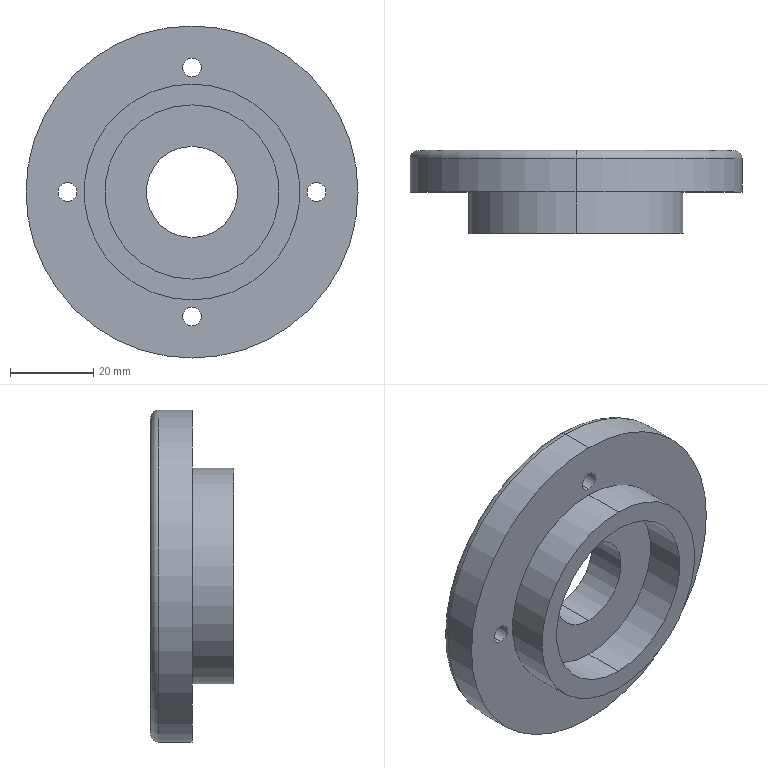Part | SolidWorks | features ICE 2, CirPattern 1, Extrusion 1, Fillet 1, HoleWzd 1 | 1 solid | 34 faces | box 80 x 20 x 80 mm | volume 52365 mm3 | cylinder 24 | plane 8 | torus 2 | commonest cylinder face diameters 4.5 x8 8 x8 22 x2 42 x2 52 x2 80 x2
STEP:
#1=CARTESIAN_POINT('',(-30.,15.4,-4.));
#2=VERTEX_POINT('',#1);
#3=CARTESIAN_POINT('',(-30.,15.4,4.));
#4=VERTEX_POINT('',#3);
#5=CARTESIAN_POINT('',(-30.,15.4,0.));
#6=DIRECTION('',(0.,1.,0.));
#7=DIRECTION('',(0.,0.,1.));
#8=AXIS2_PLACEMENT_3D('',#5,#6,#7);
#9=CIRCLE('',#8,4.);
#10=EDGE_CURVE('',#2,#4,#9,.T.);
#11=ORIENTED_EDGE('',*,*,#10,.F.);
#12=CARTESIAN_POINT('',(-30.,20.,-4.));
#13=VERTEX_POINT('',#12);
#14=CARTESIAN_POINT('',(-30.,20.,-4.));
#15=DIRECTION('',(0.,1.,0.));
#16=VECTOR('',#15,1000.);
#17=LINE('',#14,#16);
#18=EDGE_CURVE('',#2,#13,#17,.T.);
#19=ORIENTED_EDGE('',*,*,#18,.T.);
#20=CARTESIAN_POINT('',(-30.,20.,4.));
#21=VERTEX_POINT('',#20);
#22=CARTESIAN_POINT('',(-30.,20.,0.));
#23=DIRECTION('',(0.,1.,0.));
#24=DIRECTION('',(0.,0.,1.));
#25=AXIS2_PLACEMENT_3D('',#22,#23,#24);
#26=CIRCLE('',#25,4.);
#27=EDGE_CURVE('',#13,#21,#26,.T.);
#28=ORIENTED_EDGE('',*,*,#27,.T.);
#29=CARTESIAN_POINT('',(-30.,20.,4.));
#30=DIRECTION('',(0.,1.,0.));
#31=VECTOR('',#30,1000.);
#32=LINE('',#29,#31);
#33=EDGE_CURVE('',#4,#21,#32,.T.);
#34=ORIENTED_EDGE('',*,*,#33,.F.);
#35=EDGE_LOOP('',(#11,#19,#28,#34));
#36=FACE_OUTER_BOUND('',#35,.T.);
#37=CARTESIAN_POINT('',(-30.,20.,0.));
#38=DIRECTION('',(0.,1.,0.));
#39=DIRECTION('',(0.,0.,1.));
#40=AXIS2_PLACEMENT_3D('',#37,#38,#39);
#41=CYLINDRICAL_SURFACE('',#40,4.);
#42=ADVANCED_FACE('',(#36),#41,.F.);
#43=CARTESIAN_POINT('',(-30.,10.,-2.25));
#44=VERTEX_POINT('',#43);
#45=CARTESIAN_POINT('',(-30.,10.,2.25));
#46=VERTEX_POINT('',#45);
#47=CARTESIAN_POINT('',(-30.,10.,0.));
#48=DIRECTION('',(0.,1.,0.));
#49=DIRECTION('',(0.,0.,1.));
#50=AXIS2_PLACEMENT_3D('',#47,#48,#49);
#51=CIRCLE('',#50,2.25);
#52=EDGE_CURVE('',#44,#46,#51,.T.);
#53=ORIENTED_EDGE('',*,*,#52,.F.);
#54=CARTESIAN_POINT('',(-30.,15.4,-2.25));
#55=VERTEX_POINT('',#54);
#56=CARTESIAN_POINT('',(-30.,20.,-2.25));
#57=DIRECTION('',(0.,1.,0.));
#58=VECTOR('',#57,1000.);
#59=LINE('',#56,#58);
#60=EDGE_CURVE('',#44,#55,#59,.T.);
#61=ORIENTED_EDGE('',*,*,#60,.T.);
#62=CARTESIAN_POINT('',(-30.,15.4,2.25));
#63=VERTEX_POINT('',#62);
#64=CARTESIAN_POINT('',(-30.,15.4,0.));
#65=DIRECTION('',(0.,1.,0.));
#66=DIRECTION('',(0.,0.,1.));
#67=AXIS2_PLACEMENT_3D('',#64,#65,#66);
#68=CIRCLE('',#67,2.25);
#69=EDGE_CURVE('',#55,#63,#68,.T.);
#70=ORIENTED_EDGE('',*,*,#69,.T.);
#71=CARTESIAN_POINT('',(-30.,20.,2.25));
#72=DIRECTION('',(0.,1.,0.));
#73=VECTOR('',#72,1000.);
#74=LINE('',#71,#73);
#75=EDGE_CURVE('',#46,#63,#74,.T.);
#76=ORIENTED_EDGE('',*,*,#75,.F.);
#77=EDGE_LOOP('',(#53,#61,#70,#76));
#78=FACE_OUTER_BOUND('',#77,.T.);
#79=CARTESIAN_POINT('',(-30.,20.,0.));
#80=DIRECTION('',(0.,1.,0.));
#81=DIRECTION('',(0.,0.,1.));
#82=AXIS2_PLACEMENT_3D('',#79,#80,#81);
#83=CYLINDRICAL_SURFACE('',#82,2.25);
#84=ADVANCED_FACE('',(#78),#83,.F.);
#85=CARTESIAN_POINT('',(0.,15.4,26.));
#86=VERTEX_POINT('',#85);
#87=CARTESIAN_POINT('',(0.,15.4,34.));
#88=VERTEX_POINT('',#87);
#89=CARTESIAN_POINT('',(0.,15.4,30.));
#90=DIRECTION('',(0.,1.,0.));
#91=DIRECTION('',(0.,0.,1.));
#92=AXIS2_PLACEMENT_3D('',#89,#90,#91);
#93=CIRCLE('',#92,4.);
#94=EDGE_CURVE('',#86,#88,#93,.T.);
#95=ORIENTED_EDGE('',*,*,#94,.F.);
#96=CARTESIAN_POINT('',(0.,20.,26.));
#97=VERTEX_POINT('',#96);
#98=CARTESIAN_POINT('',(0.,20.,26.));
#99=DIRECTION('',(0.,1.,0.));
#100=VECTOR('',#99,1000.);
#101=LINE('',#98,#100);
#102=EDGE_CURVE('',#86,#97,#101,.T.);
#103=ORIENTED_EDGE('',*,*,#102,.T.);
#104=CARTESIAN_POINT('',(0.,20.,34.));
#105=VERTEX_POINT('',#104);
#106=CARTESIAN_POINT('',(0.,20.,30.));
#107=DIRECTION('',(0.,1.,0.));
#108=DIRECTION('',(0.,0.,1.));
#109=AXIS2_PLACEMENT_3D('',#106,#107,#108);
#110=CIRCLE('',#109,4.);
#111=EDGE_CURVE('',#97,#105,#110,.T.);
#112=ORIENTED_EDGE('',*,*,#111,.T.);
#113=CARTESIAN_POINT('',(0.,20.,34.));
#114=DIRECTION('',(0.,1.,0.));
#115=VECTOR('',#114,1000.);
#116=LINE('',#113,#115);
#117=EDGE_CURVE('',#88,#105,#116,.T.);
#118=ORIENTED_EDGE('',*,*,#117,.F.);
#119=EDGE_LOOP('',(#95,#103,#112,#118));
#120=FACE_OUTER_BOUND('',#119,.T.);
#121=CARTESIAN_POINT('',(0.,20.,30.));
#122=DIRECTION('',(0.,1.,0.));
#123=DIRECTION('',(0.,0.,1.));
#124=AXIS2_PLACEMENT_3D('',#121,#122,#123);
#125=CYLINDRICAL_SURFACE('',#124,4.);
#126=ADVANCED_FACE('',(#120),#125,.F.);
#127=CARTESIAN_POINT('',(0.,10.,27.75));
#128=VERTEX_POINT('',#127);
#129=CARTESIAN_POINT('',(0.,10.,32.25));
#130=VERTEX_POINT('',#129);
#131=CARTESIAN_POINT('',(0.,10.,30.));
#132=DIRECTION('',(0.,1.,0.));
#133=DIRECTION('',(0.,0.,1.));
#134=AXIS2_PLACEMENT_3D('',#131,#132,#133);
#135=CIRCLE('',#134,2.25);
#136=EDGE_CURVE('',#128,#130,#135,.T.);
#137=ORIENTED_EDGE('',*,*,#136,.F.);
#138=CARTESIAN_POINT('',(0.,15.4,27.75));
#139=VERTEX_POINT('',#138);
#140=CARTESIAN_POINT('',(0.,20.,27.75));
#141=DIRECTION('',(0.,1.,0.));
#142=VECTOR('',#141,1000.);
#143=LINE('',#140,#142);
#144=EDGE_CURVE('',#128,#139,#143,.T.);
#145=ORIENTED_EDGE('',*,*,#144,.T.);
#146=CARTESIAN_POINT('',(0.,15.4,32.25));
#147=VERTEX_POINT('',#146);
#148=CARTESIAN_POINT('',(0.,15.4,30.));
#149=DIRECTION('',(0.,1.,0.));
#150=DIRECTION('',(0.,0.,1.));
#151=AXIS2_PLACEMENT_3D('',#148,#149,#150);
#152=CIRCLE('',#151,2.25);
#153=EDGE_CURVE('',#139,#147,#152,.T.);
#154=ORIENTED_EDGE('',*,*,#153,.T.);
#155=CARTESIAN_POINT('',(0.,20.,32.25));
#156=DIRECTION('',(0.,1.,0.));
#157=VECTOR('',#156,1000.);
#158=LINE('',#155,#157);
#159=EDGE_CURVE('',#130,#147,#158,.T.);
#160=ORIENTED_EDGE('',*,*,#159,.F.);
#161=EDGE_LOOP('',(#137,#145,#154,#160));
#162=FACE_OUTER_BOUND('',#161,.T.);
#163=CARTESIAN_POINT('',(0.,20.,30.));
#164=DIRECTION('',(0.,1.,0.));
#165=DIRECTION('',(0.,0.,1.));
#166=AXIS2_PLACEMENT_3D('',#163,#164,#165);
#167=CYLINDRICAL_SURFACE('',#166,2.25);
#168=ADVANCED_FACE('',(#162),#167,.F.);
#169=CARTESIAN_POINT('',(30.,15.4,-4.));
#170=VERTEX_POINT('',#169);
#171=CARTESIAN_POINT('',(30.,15.4,4.));
#172=VERTEX_POINT('',#171);
#173=CARTESIAN_POINT('',(30.,15.4,0.));
#174=DIRECTION('',(0.,1.,0.));
#175=DIRECTION('',(0.,0.,1.));
#176=AXIS2_PLACEMENT_3D('',#173,#174,#175);
#177=CIRCLE('',#176,4.);
#178=EDGE_CURVE('',#170,#172,#177,.T.);
#179=ORIENTED_EDGE('',*,*,#178,.F.);
#180=CARTESIAN_POINT('',(30.,20.,-4.));
#181=VERTEX_POINT('',#180);
#182=CARTESIAN_POINT('',(30.,20.,-4.));
#183=DIRECTION('',(0.,1.,0.));
#184=VECTOR('',#183,1000.);
#185=LINE('',#182,#184);
#186=EDGE_CURVE('',#170,#181,#185,.T.);
#187=ORIENTED_EDGE('',*,*,#186,.T.);
#188=CARTESIAN_POINT('',(30.,20.,4.));
#189=VERTEX_POINT('',#188);
#190=CARTESIAN_POINT('',(30.,20.,0.));
#191=DIRECTION('',(0.,1.,0.));
#192=DIRECTION('',(0.,0.,1.));
#193=AXIS2_PLACEMENT_3D('',#190,#191,#192);
#194=CIRCLE('',#193,4.);
#195=EDGE_CURVE('',#181,#189,#194,.T.);
#196=ORIENTED_EDGE('',*,*,#195,.T.);
#197=CARTESIAN_POINT('',(30.,20.,4.));
#198=DIRECTION('',(0.,1.,0.));
#199=VECTOR('',#198,1000.);
#200=LINE('',#197,#199);
#201=EDGE_CURVE('',#172,#189,#200,.T.);
#202=ORIENTED_EDGE('',*,*,#201,.F.);
#203=EDGE_LOOP('',(#179,#187,#196,#202));
#204=FACE_OUTER_BOUND('',#203,.T.);
#205=CARTESIAN_POINT('',(30.,20.,0.));
#206=DIRECTION('',(0.,1.,0.));
#207=DIRECTION('',(0.,0.,1.));
#208=AXIS2_PLACEMENT_3D('',#205,#206,#207);
#209=CYLINDRICAL_SURFACE('',#208,4.);
#210=ADVANCED_FACE('',(#204),#209,.F.);
#211=CARTESIAN_POINT('',(30.,10.,-2.25));
#212=VERTEX_POINT('',#211);
#213=CARTESIAN_POINT('',(30.,10.,2.25));
#214=VERTEX_POINT('',#213);
#215=CARTESIAN_POINT('',(30.,10.,0.));
#216=DIRECTION('',(0.,1.,0.));
#217=DIRECTION('',(0.,0.,1.));
#218=AXIS2_PLACEMENT_3D('',#215,#216,#217);
#219=CIRCLE('',#218,2.25);
#220=EDGE_CURVE('',#212,#214,#219,.T.);
#221=ORIENTED_EDGE('',*,*,#220,.F.);
#222=CARTESIAN_POINT('',(30.,15.4,-2.25));
#223=VERTEX_POINT('',#222);
#224=CARTESIAN_POINT('',(30.,20.,-2.25));
#225=DIRECTION('',(0.,1.,0.));
#226=VECTOR('',#225,1000.);
#227=LINE('',#224,#226);
#228=EDGE_CURVE('',#212,#223,#227,.T.);
#229=ORIENTED_EDGE('',*,*,#228,.T.);
#230=CARTESIAN_POINT('',(30.,15.4,2.25));
#231=VERTEX_POINT('',#230);
#232=CARTESIAN_POINT('',(30.,15.4,0.));
#233=DIRECTION('',(0.,1.,0.));
#234=DIRECTION('',(0.,0.,1.));
#235=AXIS2_PLACEMENT_3D('',#232,#233,#234);
#236=CIRCLE('',#235,2.25);
#237=EDGE_CURVE('',#223,#231,#236,.T.);
#238=ORIENTED_EDGE('',*,*,#237,.T.);
#239=CARTESIAN_POINT('',(30.,20.,2.25));
#240=DIRECTION('',(0.,1.,0.));
#241=VECTOR('',#240,1000.);
#242=LINE('',#239,#241);
#243=EDGE_CURVE('',#214,#231,#242,.T.);
#244=ORIENTED_EDGE('',*,*,#243,.F.);
#245=EDGE_LOOP('',(#221,#229,#238,#244));
#246=FACE_OUTER_BOUND('',#245,.T.);
#247=CARTESIAN_POINT('',(30.,20.,0.));
#248=DIRECTION('',(0.,1.,0.));
#249=DIRECTION('',(0.,0.,1.));
#250=AXIS2_PLACEMENT_3D('',#247,#248,#249);
#251=CYLINDRICAL_SURFACE('',#250,2.25);
#252=ADVANCED_FACE('',(#246),#251,.F.);
#253=CARTESIAN_POINT('',(0.,15.4,-34.));
#254=VERTEX_POINT('',#253);
#255=CARTESIAN_POINT('',(0.,15.4,-26.));
#256=VERTEX_POINT('',#255);
#257=CARTESIAN_POINT('',(0.,15.4,-30.));
#258=DIRECTION('',(0.,1.,0.));
#259=DIRECTION('',(0.,0.,1.));
#260=AXIS2_PLACEMENT_3D('',#257,#258,#259);
#261=CIRCLE('',#260,4.);
#262=EDGE_CURVE('',#254,#256,#261,.T.);
#263=ORIENTED_EDGE('',*,*,#262,.F.);
#264=CARTESIAN_POINT('',(0.,20.,-34.));
#265=VERTEX_POINT('',#264);
#266=CARTESIAN_POINT('',(0.,20.,-34.));
#267=DIRECTION('',(0.,1.,0.));
#268=VECTOR('',#267,1000.);
#269=LINE('',#266,#268);
#270=EDGE_CURVE('',#254,#265,#269,.T.);
#271=ORIENTED_EDGE('',*,*,#270,.T.);
#272=CARTESIAN_POINT('',(0.,20.,-26.));
#273=VERTEX_POINT('',#272);
#274=CARTESIAN_POINT('',(0.,20.,-30.));
#275=DIRECTION('',(0.,1.,0.));
#276=DIRECTION('',(0.,0.,1.));
#277=AXIS2_PLACEMENT_3D('',#274,#275,#276);
#278=CIRCLE('',#277,4.);
#279=EDGE_CURVE('',#265,#273,#278,.T.);
#280=ORIENTED_EDGE('',*,*,#279,.T.);
#281=CARTESIAN_POINT('',(0.,20.,-26.));
#282=DIRECTION('',(0.,1.,0.));
#283=VECTOR('',#282,1000.);
#284=LINE('',#281,#283);
#285=EDGE_CURVE('',#256,#273,#284,.T.);
#286=ORIENTED_EDGE('',*,*,#285,.F.);
#287=EDGE_LOOP('',(#263,#271,#280,#286));
#288=FACE_OUTER_BOUND('',#287,.T.);
#289=CARTESIAN_POINT('',(0.,20.,-30.));
#290=DIRECTION('',(0.,1.,0.));
#291=DIRECTION('',(0.,0.,1.));
#292=AXIS2_PLACEMENT_3D('',#289,#290,#291);
#293=CYLINDRICAL_SURFACE('',#292,4.);
#294=ADVANCED_FACE('',(#288),#293,.F.);
#295=CARTESIAN_POINT('',(0.,10.,-32.25));
#296=VERTEX_POINT('',#295);
#297=CARTESIAN_POINT('',(0.,10.,-27.75));
#298=VERTEX_POINT('',#297);
#299=CARTESIAN_POINT('',(0.,10.,-30.));
#300=DIRECTION('',(0.,1.,0.));
#301=DIRECTION('',(0.,0.,1.));
#302=AXIS2_PLACEMENT_3D('',#299,#300,#301);
#303=CIRCLE('',#302,2.25);
#304=EDGE_CURVE('',#296,#298,#303,.T.);
#305=ORIENTED_EDGE('',*,*,#304,.F.);
#306=CARTESIAN_POINT('',(0.,15.4,-32.25));
#307=VERTEX_POINT('',#306);
#308=CARTESIAN_POINT('',(0.,20.,-32.25));
#309=DIRECTION('',(0.,1.,0.));
#310=VECTOR('',#309,1000.);
#311=LINE('',#308,#310);
#312=EDGE_CURVE('',#296,#307,#311,.T.);
#313=ORIENTED_EDGE('',*,*,#312,.T.);
#314=CARTESIAN_POINT('',(0.,15.4,-27.75));
#315=VERTEX_POINT('',#314);
#316=CARTESIAN_POINT('',(0.,15.4,-30.));
#317=DIRECTION('',(0.,1.,0.));
#318=DIRECTION('',(0.,0.,1.));
#319=AXIS2_PLACEMENT_3D('',#316,#317,#318);
#320=CIRCLE('',#319,2.25);
#321=EDGE_CURVE('',#307,#315,#320,.T.);
#322=ORIENTED_EDGE('',*,*,#321,.T.);
#323=CARTESIAN_POINT('',(0.,20.,-27.75));
#324=DIRECTION('',(0.,1.,0.));
#325=VECTOR('',#324,1000.);
#326=LINE('',#323,#325);
#327=EDGE_CURVE('',#298,#315,#326,.T.);
#328=ORIENTED_EDGE('',*,*,#327,.F.);
#329=EDGE_LOOP('',(#305,#313,#322,#328));
#330=FACE_OUTER_BOUND('',#329,.T.);
#331=CARTESIAN_POINT('',(0.,20.,-30.));
#332=DIRECTION('',(0.,1.,0.));
#333=DIRECTION('',(0.,0.,1.));
#334=AXIS2_PLACEMENT_3D('',#331,#332,#333);
#335=CYLINDRICAL_SURFACE('',#334,2.25);
#336=ADVANCED_FACE('',(#330),#335,.F.);
#337=CARTESIAN_POINT('',(0.,18.,-40.));
#338=VERTEX_POINT('',#337);
#339=CARTESIAN_POINT('',(0.,18.,40.));
#340=VERTEX_POINT('',#339);
#341=CARTESIAN_POINT('',(0.,18.,0.));
#342=DIRECTION('',(0.,-1.,0.));
#343=DIRECTION('',(0.,0.,1.));
#344=AXIS2_PLACEMENT_3D('',#341,#342,#343);
#345=CIRCLE('',#344,40.);
#346=EDGE_CURVE('',#338,#340,#345,.T.);
#347=ORIENTED_EDGE('',*,*,#346,.F.);
#348=CARTESIAN_POINT('',(0.,20.,-38.));
#349=VERTEX_POINT('',#348);
#350=CARTESIAN_POINT('',(0.,18.,-38.));
#351=DIRECTION('',(1.,0.,0.));
#352=DIRECTION('',(0.,0.,-1.));
#353=AXIS2_PLACEMENT_3D('',#350,#351,#352);
#354=CIRCLE('',#353,2.);
#355=EDGE_CURVE('',#338,#349,#354,.T.);
#356=ORIENTED_EDGE('',*,*,#355,.T.);
#357=CARTESIAN_POINT('',(0.,20.,38.));
#358=VERTEX_POINT('',#357);
#359=CARTESIAN_POINT('',(0.,20.,0.));
#360=DIRECTION('',(0.,1.,0.));
#361=DIRECTION('',(0.,0.,1.));
#362=AXIS2_PLACEMENT_3D('',#359,#360,#361);
#363=CIRCLE('',#362,38.);
#364=EDGE_CURVE('',#358,#349,#363,.T.);
#365=ORIENTED_EDGE('',*,*,#364,.F.);
#366=CARTESIAN_POINT('',(0.,18.,38.));
#367=DIRECTION('',(-1.,0.,0.));
#368=DIRECTION('',(0.,0.,1.));
#369=AXIS2_PLACEMENT_3D('',#366,#367,#368);
#370=CIRCLE('',#369,2.);
#371=EDGE_CURVE('',#340,#358,#370,.T.);
#372=ORIENTED_EDGE('',*,*,#371,.F.);
#373=EDGE_LOOP('',(#347,#356,#365,#372));
#374=FACE_OUTER_BOUND('',#373,.T.);
#375=CARTESIAN_POINT('',(0.,18.,0.));
#376=DIRECTION('',(0.,1.,0.));
#377=DIRECTION('',(0.,0.,1.));
#378=AXIS2_PLACEMENT_3D('',#375,#376,#377);
#379=TOROIDAL_SURFACE('',#378,38.,2.);
#380=ADVANCED_FACE('',(#374),#379,.T.);
#381=CARTESIAN_POINT('',(0.,20.,11.));
#382=VERTEX_POINT('',#381);
#383=CARTESIAN_POINT('',(0.,20.,-11.));
#384=VERTEX_POINT('',#383);
#385=CARTESIAN_POINT('',(0.,20.,0.));
#386=DIRECTION('',(0.,-1.,0.));
#387=DIRECTION('',(0.,0.,-1.));
#388=AXIS2_PLACEMENT_3D('',#385,#386,#387);
#389=CIRCLE('',#388,11.);
#390=EDGE_CURVE('',#382,#384,#389,.T.);
#391=ORIENTED_EDGE('',*,*,#390,.F.);
#392=CARTESIAN_POINT('',(0.,10.,11.));
#393=VERTEX_POINT('',#392);
#394=CARTESIAN_POINT('',(0.,20.,11.));
#395=DIRECTION('',(0.,-1.,0.));
#396=VECTOR('',#395,1000.);
#397=LINE('',#394,#396);
#398=EDGE_CURVE('',#382,#393,#397,.T.);
#399=ORIENTED_EDGE('',*,*,#398,.T.);
#400=CARTESIAN_POINT('',(0.,10.,-11.));
#401=VERTEX_POINT('',#400);
#402=CARTESIAN_POINT('',(0.,10.,0.));
#403=DIRECTION('',(0.,-1.,0.));
#404=DIRECTION('',(0.,0.,-1.));
#405=AXIS2_PLACEMENT_3D('',#402,#403,#404);
#406=CIRCLE('',#405,11.);
#407=EDGE_CURVE('',#393,#401,#406,.T.);
#408=ORIENTED_EDGE('',*,*,#407,.T.);
#409=CARTESIAN_POINT('',(0.,20.,-11.));
#410=DIRECTION('',(0.,-1.,0.));
#411=VECTOR('',#410,1000.);
#412=LINE('',#409,#411);
#413=EDGE_CURVE('',#384,#401,#412,.T.);
#414=ORIENTED_EDGE('',*,*,#413,.F.);
#415=EDGE_LOOP('',(#391,#399,#408,#414));
#416=FACE_OUTER_BOUND('',#415,.T.);
#417=CARTESIAN_POINT('',(0.,20.,0.));
#418=DIRECTION('',(0.,-1.,0.));
#419=DIRECTION('',(0.,0.,-1.));
#420=AXIS2_PLACEMENT_3D('',#417,#418,#419);
#421=CYLINDRICAL_SURFACE('',#420,11.);
#422=ADVANCED_FACE('',(#416),#421,.F.);
#423=ORIENTED_EDGE('',*,*,#346,.T.);
#424=CARTESIAN_POINT('',(0.,10.,40.));
#425=VERTEX_POINT('',#424);
#426=CARTESIAN_POINT('',(0.,20.,40.));
#427=DIRECTION('',(0.,-1.,0.));
#428=VECTOR('',#427,1000.);
#429=LINE('',#426,#428);
#430=EDGE_CURVE('',#340,#425,#429,.T.);
#431=ORIENTED_EDGE('',*,*,#430,.T.);
#432=CARTESIAN_POINT('',(0.,10.,-40.));
#433=VERTEX_POINT('',#432);
#434=CARTESIAN_POINT('',(0.,10.,0.));
#435=DIRECTION('',(0.,1.,0.));
#436=DIRECTION('',(0.,0.,1.));
#437=AXIS2_PLACEMENT_3D('',#434,#435,#436);
#438=CIRCLE('',#437,40.);
#439=EDGE_CURVE('',#425,#433,#438,.T.);
#440=ORIENTED_EDGE('',*,*,#439,.T.);
#441=CARTESIAN_POINT('',(0.,20.,-40.));
#442=DIRECTION('',(0.,-1.,0.));
#443=VECTOR('',#442,1000.);
#444=LINE('',#441,#443);
#445=EDGE_CURVE('',#338,#433,#444,.T.);
#446=ORIENTED_EDGE('',*,*,#445,.F.);
#447=EDGE_LOOP('',(#423,#431,#440,#446));
#448=FACE_OUTER_BOUND('',#447,.T.);
#449=CARTESIAN_POINT('',(0.,20.,0.));
#450=DIRECTION('',(0.,-1.,0.));
#451=DIRECTION('',(0.,0.,-1.));
#452=AXIS2_PLACEMENT_3D('',#449,#450,#451);
#453=CYLINDRICAL_SURFACE('',#452,40.);
#454=ADVANCED_FACE('',(#448),#453,.T.);
#455=CARTESIAN_POINT('',(0.,10.,-21.));
#456=VERTEX_POINT('',#455);
#457=CARTESIAN_POINT('',(0.,10.,21.));
#458=VERTEX_POINT('',#457);
#459=CARTESIAN_POINT('',(0.,10.,0.));
#460=DIRECTION('',(0.,1.,0.));
#461=DIRECTION('',(0.,0.,1.));
#462=AXIS2_PLACEMENT_3D('',#459,#460,#461);
#463=CIRCLE('',#462,21.);
#464=EDGE_CURVE('',#456,#458,#463,.T.);
#465=ORIENTED_EDGE('',*,*,#464,.T.);
#466=CARTESIAN_POINT('',(0.,0.,21.));
#467=VERTEX_POINT('',#466);
#468=CARTESIAN_POINT('',(0.,10.,21.));
#469=DIRECTION('',(0.,-1.,0.));
#470=VECTOR('',#469,1000.);
#471=LINE('',#468,#470);
#472=EDGE_CURVE('',#458,#467,#471,.T.);
#473=ORIENTED_EDGE('',*,*,#472,.T.);
#474=CARTESIAN_POINT('',(0.,0.,-21.));
#475=VERTEX_POINT('',#474);
#476=CARTESIAN_POINT('',(0.,0.,0.));
#477=DIRECTION('',(0.,1.,0.));
#478=DIRECTION('',(0.,0.,1.));
#479=AXIS2_PLACEMENT_3D('',#476,#477,#478);
#480=CIRCLE('',#479,21.);
#481=EDGE_CURVE('',#475,#467,#480,.T.);
#482=ORIENTED_EDGE('',*,*,#481,.F.);
#483=CARTESIAN_POINT('',(0.,10.,-21.));
#484=DIRECTION('',(0.,-1.,0.));
#485=VECTOR('',#484,1000.);
#486=LINE('',#483,#485);
#487=EDGE_CURVE('',#456,#475,#486,.T.);
#488=ORIENTED_EDGE('',*,*,#487,.F.);
#489=EDGE_LOOP('',(#465,#473,#482,#488));
#490=FACE_OUTER_BOUND('',#489,.T.);
#491=CARTESIAN_POINT('',(0.,10.,0.));
#492=DIRECTION('',(0.,-1.,0.));
#493=DIRECTION('',(0.,0.,-1.));
#494=AXIS2_PLACEMENT_3D('',#491,#492,#493);
#495=CYLINDRICAL_SURFACE('',#494,21.);
#496=ADVANCED_FACE('',(#490),#495,.F.);
#497=CARTESIAN_POINT('',(0.,10.,26.));
#498=VERTEX_POINT('',#497);
#499=CARTESIAN_POINT('',(0.,10.,-26.));
#500=VERTEX_POINT('',#499);
#501=CARTESIAN_POINT('',(0.,10.,0.));
#502=DIRECTION('',(0.,1.,0.));
#503=DIRECTION('',(0.,0.,1.));
#504=AXIS2_PLACEMENT_3D('',#501,#502,#503);
#505=CIRCLE('',#504,26.);
#506=EDGE_CURVE('',#498,#500,#505,.T.);
#507=ORIENTED_EDGE('',*,*,#506,.F.);
#508=CARTESIAN_POINT('',(0.,0.,26.));
#509=VERTEX_POINT('',#508);
#510=CARTESIAN_POINT('',(0.,10.,26.));
#511=DIRECTION('',(0.,-1.,0.));
#512=VECTOR('',#511,1000.);
#513=LINE('',#510,#512);
#514=EDGE_CURVE('',#498,#509,#513,.T.);
#515=ORIENTED_EDGE('',*,*,#514,.T.);
#516=CARTESIAN_POINT('',(0.,0.,-26.));
#517=VERTEX_POINT('',#516);
#518=CARTESIAN_POINT('',(0.,0.,0.));
#519=DIRECTION('',(0.,1.,0.));
#520=DIRECTION('',(0.,0.,1.));
#521=AXIS2_PLACEMENT_3D('',#518,#519,#520);
#522=CIRCLE('',#521,26.);
#523=EDGE_CURVE('',#509,#517,#522,.T.);
#524=ORIENTED_EDGE('',*,*,#523,.T.);
#525=CARTESIAN_POINT('',(0.,10.,-26.));
#526=DIRECTION('',(0.,-1.,0.));
#527=VECTOR('',#526,1000.);
#528=LINE('',#525,#527);
#529=EDGE_CURVE('',#500,#517,#528,.T.);
#530=ORIENTED_EDGE('',*,*,#529,.F.);
#531=EDGE_LOOP('',(#507,#515,#524,#530));
#532=FACE_OUTER_BOUND('',#531,.T.);
#533=CARTESIAN_POINT('',(0.,10.,0.));
#534=DIRECTION('',(0.,-1.,0.));
#535=DIRECTION('',(0.,0.,-1.));
#536=AXIS2_PLACEMENT_3D('',#533,#534,#535);
#537=CYLINDRICAL_SURFACE('',#536,26.);
#538=ADVANCED_FACE('',(#532),#537,.T.);
#539=CARTESIAN_POINT('',(0.,0.,0.));
#540=DIRECTION('',(0.,1.,0.));
#541=DIRECTION('',(0.,0.,1.));
#542=AXIS2_PLACEMENT_3D('',#539,#540,#541);
#543=CIRCLE('',#542,26.);
#544=EDGE_CURVE('',#517,#509,#543,.T.);
#545=ORIENTED_EDGE('',*,*,#544,.F.);
#546=ORIENTED_EDGE('',*,*,#523,.F.);
#547=EDGE_LOOP('',(#545,#546));
#548=FACE_OUTER_BOUND('',#547,.T.);
#549=ORIENTED_EDGE('',*,*,#481,.T.);
#550=CARTESIAN_POINT('',(0.,0.,0.));
#551=DIRECTION('',(0.,1.,0.));
#552=DIRECTION('',(0.,0.,1.));
#553=AXIS2_PLACEMENT_3D('',#550,#551,#552);
#554=CIRCLE('',#553,21.);
#555=EDGE_CURVE('',#467,#475,#554,.T.);
#556=ORIENTED_EDGE('',*,*,#555,.T.);
#557=EDGE_LOOP('',(#549,#556));
#558=FACE_BOUND('',#557,.T.);
#559=CARTESIAN_POINT('',(0.,0.,0.));
#560=DIRECTION('',(0.,1.,0.));
#561=DIRECTION('',(0.,0.,1.));
#562=AXIS2_PLACEMENT_3D('',#559,#560,#561);
#563=PLANE('',#562);
#564=ADVANCED_FACE('',(#548,#558),#563,.F.);
#565=ORIENTED_EDGE('',*,*,#514,.F.);
#566=CARTESIAN_POINT('',(0.,10.,0.));
#567=DIRECTION('',(0.,1.,0.));
#568=DIRECTION('',(0.,0.,1.));
#569=AXIS2_PLACEMENT_3D('',#566,#567,#568);
#570=CIRCLE('',#569,26.);
#571=EDGE_CURVE('',#500,#498,#570,.T.);
#572=ORIENTED_EDGE('',*,*,#571,.F.);
#573=ORIENTED_EDGE('',*,*,#529,.T.);
#574=ORIENTED_EDGE('',*,*,#544,.T.);
#575=EDGE_LOOP('',(#565,#572,#573,#574));
#576=FACE_OUTER_BOUND('',#575,.T.);
#577=CARTESIAN_POINT('',(0.,10.,0.));
#578=DIRECTION('',(0.,-1.,0.));
#579=DIRECTION('',(0.,0.,-1.));
#580=AXIS2_PLACEMENT_3D('',#577,#578,#579);
#581=CYLINDRICAL_SURFACE('',#580,26.);
#582=ADVANCED_FACE('',(#576),#581,.T.);
#583=ORIENTED_EDGE('',*,*,#472,.F.);
#584=CARTESIAN_POINT('',(0.,10.,0.));
#585=DIRECTION('',(0.,1.,0.));
#586=DIRECTION('',(0.,0.,1.));
#587=AXIS2_PLACEMENT_3D('',#584,#585,#586);
#588=CIRCLE('',#587,21.);
#589=EDGE_CURVE('',#458,#456,#588,.T.);
#590=ORIENTED_EDGE('',*,*,#589,.T.);
#591=ORIENTED_EDGE('',*,*,#487,.T.);
#592=ORIENTED_EDGE('',*,*,#555,.F.);
#593=EDGE_LOOP('',(#583,#590,#591,#592));
#594=FACE_OUTER_BOUND('',#593,.T.);
#595=CARTESIAN_POINT('',(0.,10.,0.));
#596=DIRECTION('',(0.,-1.,0.));
#597=DIRECTION('',(0.,0.,-1.));
#598=AXIS2_PLACEMENT_3D('',#595,#596,#597);
#599=CYLINDRICAL_SURFACE('',#598,21.);
#600=ADVANCED_FACE('',(#594),#599,.F.);
#601=CARTESIAN_POINT('',(0.,10.,0.));
#602=DIRECTION('',(0.,-1.,0.));
#603=DIRECTION('',(0.,0.,-1.));
#604=AXIS2_PLACEMENT_3D('',#601,#602,#603);
#605=CIRCLE('',#604,11.);
#606=EDGE_CURVE('',#401,#393,#605,.T.);
#607=ORIENTED_EDGE('',*,*,#606,.F.);
#608=ORIENTED_EDGE('',*,*,#407,.F.);
#609=EDGE_LOOP('',(#607,#608));
#610=FACE_BOUND('',#609,.T.);
#611=ORIENTED_EDGE('',*,*,#464,.F.);
#612=ORIENTED_EDGE('',*,*,#589,.F.);
#613=EDGE_LOOP('',(#611,#612));
#614=FACE_OUTER_BOUND('',#613,.T.);
#615=CARTESIAN_POINT('',(0.,10.,0.));
#616=DIRECTION('',(0.,1.,0.));
#617=DIRECTION('',(0.,0.,1.));
#618=AXIS2_PLACEMENT_3D('',#615,#616,#617);
#619=PLANE('',#618);
#620=ADVANCED_FACE('',(#610,#614),#619,.F.);
#621=ORIENTED_EDGE('',*,*,#430,.F.);
#622=CARTESIAN_POINT('',(0.,18.,0.));
#623=DIRECTION('',(0.,-1.,0.));
#624=DIRECTION('',(0.,0.,1.));
#625=AXIS2_PLACEMENT_3D('',#622,#623,#624);
#626=CIRCLE('',#625,40.);
#627=EDGE_CURVE('',#340,#338,#626,.T.);
#628=ORIENTED_EDGE('',*,*,#627,.T.);
#629=ORIENTED_EDGE('',*,*,#445,.T.);
#630=CARTESIAN_POINT('',(0.,10.,0.));
#631=DIRECTION('',(0.,1.,0.));
#632=DIRECTION('',(0.,0.,1.));
#633=AXIS2_PLACEMENT_3D('',#630,#631,#632);
#634=CIRCLE('',#633,40.);
#635=EDGE_CURVE('',#433,#425,#634,.T.);
#636=ORIENTED_EDGE('',*,*,#635,.T.);
#637=EDGE_LOOP('',(#621,#628,#629,#636));
#638=FACE_OUTER_BOUND('',#637,.T.);
#639=CARTESIAN_POINT('',(0.,20.,0.));
#640=DIRECTION('',(0.,-1.,0.));
#641=DIRECTION('',(0.,0.,-1.));
#642=AXIS2_PLACEMENT_3D('',#639,#640,#641);
#643=CYLINDRICAL_SURFACE('',#642,40.);
#644=ADVANCED_FACE('',(#638),#643,.T.);
#645=CARTESIAN_POINT('',(-30.,20.,0.));
#646=DIRECTION('',(0.,1.,0.));
#647=DIRECTION('',(0.,0.,1.));
#648=AXIS2_PLACEMENT_3D('',#645,#646,#647);
#649=CIRCLE('',#648,4.);
#650=EDGE_CURVE('',#21,#13,#649,.T.);
#651=ORIENTED_EDGE('',*,*,#650,.F.);
#652=ORIENTED_EDGE('',*,*,#27,.F.);
#653=EDGE_LOOP('',(#651,#652));
#654=FACE_BOUND('',#653,.T.);
#655=CARTESIAN_POINT('',(0.,20.,30.));
#656=DIRECTION('',(0.,1.,0.));
#657=DIRECTION('',(0.,0.,1.));
#658=AXIS2_PLACEMENT_3D('',#655,#656,#657);
#659=CIRCLE('',#658,4.);
#660=EDGE_CURVE('',#105,#97,#659,.T.);
#661=ORIENTED_EDGE('',*,*,#660,.F.);
#662=ORIENTED_EDGE('',*,*,#111,.F.);
#663=EDGE_LOOP('',(#661,#662));
#664=FACE_BOUND('',#663,.T.);
#665=CARTESIAN_POINT('',(30.,20.,0.));
#666=DIRECTION('',(0.,1.,0.));
#667=DIRECTION('',(0.,0.,1.));
#668=AXIS2_PLACEMENT_3D('',#665,#666,#667);
#669=CIRCLE('',#668,4.);
#670=EDGE_CURVE('',#189,#181,#669,.T.);
#671=ORIENTED_EDGE('',*,*,#670,.F.);
#672=ORIENTED_EDGE('',*,*,#195,.F.);
#673=EDGE_LOOP('',(#671,#672));
#674=FACE_BOUND('',#673,.T.);
#675=CARTESIAN_POINT('',(0.,20.,-30.));
#676=DIRECTION('',(0.,1.,0.));
#677=DIRECTION('',(0.,0.,1.));
#678=AXIS2_PLACEMENT_3D('',#675,#676,#677);
#679=CIRCLE('',#678,4.);
#680=EDGE_CURVE('',#273,#265,#679,.T.);
#681=ORIENTED_EDGE('',*,*,#680,.F.);
#682=ORIENTED_EDGE('',*,*,#279,.F.);
#683=EDGE_LOOP('',(#681,#682));
#684=FACE_BOUND('',#683,.T.);
#685=ORIENTED_EDGE('',*,*,#364,.T.);
#686=CARTESIAN_POINT('',(0.,20.,0.));
#687=DIRECTION('',(0.,1.,0.));
#688=DIRECTION('',(0.,0.,1.));
#689=AXIS2_PLACEMENT_3D('',#686,#687,#688);
#690=CIRCLE('',#689,38.);
#691=EDGE_CURVE('',#349,#358,#690,.T.);
#692=ORIENTED_EDGE('',*,*,#691,.T.);
#693=EDGE_LOOP('',(#685,#692));
#694=FACE_OUTER_BOUND('',#693,.T.);
#695=CARTESIAN_POINT('',(0.,20.,0.));
#696=DIRECTION('',(0.,-1.,0.));
#697=DIRECTION('',(0.,0.,-1.));
#698=AXIS2_PLACEMENT_3D('',#695,#696,#697);
#699=CIRCLE('',#698,11.);
#700=EDGE_CURVE('',#384,#382,#699,.T.);
#701=ORIENTED_EDGE('',*,*,#700,.T.);
#702=ORIENTED_EDGE('',*,*,#390,.T.);
#703=EDGE_LOOP('',(#701,#702));
#704=FACE_BOUND('',#703,.T.);
#705=CARTESIAN_POINT('',(0.,20.,0.));
#706=DIRECTION('',(0.,1.,0.));
#707=DIRECTION('',(0.,0.,1.));
#708=AXIS2_PLACEMENT_3D('',#705,#706,#707);
#709=PLANE('',#708);
#710=ADVANCED_FACE('',(#654,#664,#674,#684,#694,#704),#709,.T.);
#711=CARTESIAN_POINT('',(-30.,10.,0.));
#712=DIRECTION('',(0.,1.,0.));
#713=DIRECTION('',(0.,0.,1.));
#714=AXIS2_PLACEMENT_3D('',#711,#712,#713);
#715=CIRCLE('',#714,2.25);
#716=EDGE_CURVE('',#46,#44,#715,.T.);
#717=ORIENTED_EDGE('',*,*,#716,.T.);
#718=ORIENTED_EDGE('',*,*,#52,.T.);
#719=EDGE_LOOP('',(#717,#718));
#720=FACE_BOUND('',#719,.T.);
#721=CARTESIAN_POINT('',(0.,10.,30.));
#722=DIRECTION('',(0.,1.,0.));
#723=DIRECTION('',(0.,0.,1.));
#724=AXIS2_PLACEMENT_3D('',#721,#722,#723);
#725=CIRCLE('',#724,2.25);
#726=EDGE_CURVE('',#130,#128,#725,.T.);
#727=ORIENTED_EDGE('',*,*,#726,.T.);
#728=ORIENTED_EDGE('',*,*,#136,.T.);
#729=EDGE_LOOP('',(#727,#728));
#730=FACE_BOUND('',#729,.T.);
#731=CARTESIAN_POINT('',(30.,10.,0.));
#732=DIRECTION('',(0.,1.,0.));
#733=DIRECTION('',(0.,0.,1.));
#734=AXIS2_PLACEMENT_3D('',#731,#732,#733);
#735=CIRCLE('',#734,2.25);
#736=EDGE_CURVE('',#214,#212,#735,.T.);
#737=ORIENTED_EDGE('',*,*,#736,.T.);
#738=ORIENTED_EDGE('',*,*,#220,.T.);
#739=EDGE_LOOP('',(#737,#738));
#740=FACE_BOUND('',#739,.T.);
#741=CARTESIAN_POINT('',(0.,10.,-30.));
#742=DIRECTION('',(0.,1.,0.));
#743=DIRECTION('',(0.,0.,1.));
#744=AXIS2_PLACEMENT_3D('',#741,#742,#743);
#745=CIRCLE('',#744,2.25);
#746=EDGE_CURVE('',#298,#296,#745,.T.);
#747=ORIENTED_EDGE('',*,*,#746,.T.);
#748=ORIENTED_EDGE('',*,*,#304,.T.);
#749=EDGE_LOOP('',(#747,#748));
#750=FACE_BOUND('',#749,.T.);
#751=ORIENTED_EDGE('',*,*,#571,.T.);
#752=ORIENTED_EDGE('',*,*,#506,.T.);
#753=EDGE_LOOP('',(#751,#752));
#754=FACE_BOUND('',#753,.T.);
#755=ORIENTED_EDGE('',*,*,#635,.F.);
#756=ORIENTED_EDGE('',*,*,#439,.F.);
#757=EDGE_LOOP('',(#755,#756));
#758=FACE_OUTER_BOUND('',#757,.T.);
#759=CARTESIAN_POINT('',(0.,10.,0.));
#760=DIRECTION('',(0.,1.,0.));
#761=DIRECTION('',(0.,0.,1.));
#762=AXIS2_PLACEMENT_3D('',#759,#760,#761);
#763=PLANE('',#762);
#764=ADVANCED_FACE('',(#720,#730,#740,#750,#754,#758),#763,.F.);
#765=ORIENTED_EDGE('',*,*,#398,.F.);
#766=ORIENTED_EDGE('',*,*,#700,.F.);
#767=ORIENTED_EDGE('',*,*,#413,.T.);
#768=ORIENTED_EDGE('',*,*,#606,.T.);
#769=EDGE_LOOP('',(#765,#766,#767,#768));
#770=FACE_OUTER_BOUND('',#769,.T.);
#771=CARTESIAN_POINT('',(0.,20.,0.));
#772=DIRECTION('',(0.,-1.,0.));
#773=DIRECTION('',(0.,0.,-1.));
#774=AXIS2_PLACEMENT_3D('',#771,#772,#773);
#775=CYLINDRICAL_SURFACE('',#774,11.);
#776=ADVANCED_FACE('',(#770),#775,.F.);
#777=ORIENTED_EDGE('',*,*,#355,.F.);
#778=ORIENTED_EDGE('',*,*,#627,.F.);
#779=ORIENTED_EDGE('',*,*,#371,.T.);
#780=ORIENTED_EDGE('',*,*,#691,.F.);
#781=EDGE_LOOP('',(#777,#778,#779,#780));
#782=FACE_OUTER_BOUND('',#781,.T.);
#783=CARTESIAN_POINT('',(0.,18.,0.));
#784=DIRECTION('',(0.,1.,0.));
#785=DIRECTION('',(0.,0.,1.));
#786=AXIS2_PLACEMENT_3D('',#783,#784,#785);
#787=TOROIDAL_SURFACE('',#786,38.,2.);
#788=ADVANCED_FACE('',(#782),#787,.T.);
#789=ORIENTED_EDGE('',*,*,#312,.F.);
#790=ORIENTED_EDGE('',*,*,#746,.F.);
#791=ORIENTED_EDGE('',*,*,#327,.T.);
#792=CARTESIAN_POINT('',(0.,15.4,-30.));
#793=DIRECTION('',(0.,1.,0.));
#794=DIRECTION('',(0.,0.,1.));
#795=AXIS2_PLACEMENT_3D('',#792,#793,#794);
#796=CIRCLE('',#795,2.25);
#797=EDGE_CURVE('',#315,#307,#796,.T.);
#798=ORIENTED_EDGE('',*,*,#797,.T.);
#799=EDGE_LOOP('',(#789,#790,#791,#798));
#800=FACE_OUTER_BOUND('',#799,.T.);
#801=CARTESIAN_POINT('',(0.,20.,-30.));
#802=DIRECTION('',(0.,1.,0.));
#803=DIRECTION('',(0.,0.,1.));
#804=AXIS2_PLACEMENT_3D('',#801,#802,#803);
#805=CYLINDRICAL_SURFACE('',#804,2.25);
#806=ADVANCED_FACE('',(#800),#805,.F.);
#807=ORIENTED_EDGE('',*,*,#797,.F.);
#808=ORIENTED_EDGE('',*,*,#321,.F.);
#809=EDGE_LOOP('',(#807,#808));
#810=FACE_BOUND('',#809,.T.);
#811=CARTESIAN_POINT('',(0.,15.4,-30.));
#812=DIRECTION('',(0.,1.,0.));
#813=DIRECTION('',(0.,0.,1.));
#814=AXIS2_PLACEMENT_3D('',#811,#812,#813);
#815=CIRCLE('',#814,4.);
#816=EDGE_CURVE('',#256,#254,#815,.T.);
#817=ORIENTED_EDGE('',*,*,#816,.T.);
#818=ORIENTED_EDGE('',*,*,#262,.T.);
#819=EDGE_LOOP('',(#817,#818));
#820=FACE_OUTER_BOUND('',#819,.T.);
#821=CARTESIAN_POINT('',(2.25,15.4,-30.));
#822=DIRECTION('',(0.,-1.,0.));
#823=DIRECTION('',(0.,0.,-1.));
#824=AXIS2_PLACEMENT_3D('',#821,#822,#823);
#825=PLANE('',#824);
#826=ADVANCED_FACE('',(#810,#820),#825,.F.);
#827=ORIENTED_EDGE('',*,*,#270,.F.);
#828=ORIENTED_EDGE('',*,*,#816,.F.);
#829=ORIENTED_EDGE('',*,*,#285,.T.);
#830=ORIENTED_EDGE('',*,*,#680,.T.);
#831=EDGE_LOOP('',(#827,#828,#829,#830));
#832=FACE_OUTER_BOUND('',#831,.T.);
#833=CARTESIAN_POINT('',(0.,20.,-30.));
#834=DIRECTION('',(0.,1.,0.));
#835=DIRECTION('',(0.,0.,1.));
#836=AXIS2_PLACEMENT_3D('',#833,#834,#835);
#837=CYLINDRICAL_SURFACE('',#836,4.);
#838=ADVANCED_FACE('',(#832),#837,.F.);
#839=ORIENTED_EDGE('',*,*,#228,.F.);
#840=ORIENTED_EDGE('',*,*,#736,.F.);
#841=ORIENTED_EDGE('',*,*,#243,.T.);
#842=CARTESIAN_POINT('',(30.,15.4,0.));
#843=DIRECTION('',(0.,1.,0.));
#844=DIRECTION('',(0.,0.,1.));
#845=AXIS2_PLACEMENT_3D('',#842,#843,#844);
#846=CIRCLE('',#845,2.25);
#847=EDGE_CURVE('',#231,#223,#846,.T.);
#848=ORIENTED_EDGE('',*,*,#847,.T.);
#849=EDGE_LOOP('',(#839,#840,#841,#848));
#850=FACE_OUTER_BOUND('',#849,.T.);
#851=CARTESIAN_POINT('',(30.,20.,0.));
#852=DIRECTION('',(0.,1.,0.));
#853=DIRECTION('',(0.,0.,1.));
#854=AXIS2_PLACEMENT_3D('',#851,#852,#853);
#855=CYLINDRICAL_SURFACE('',#854,2.25);
#856=ADVANCED_FACE('',(#850),#855,.F.);
#857=ORIENTED_EDGE('',*,*,#847,.F.);
#858=ORIENTED_EDGE('',*,*,#237,.F.);
#859=EDGE_LOOP('',(#857,#858));
#860=FACE_BOUND('',#859,.T.);
#861=CARTESIAN_POINT('',(30.,15.4,0.));
#862=DIRECTION('',(0.,1.,0.));
#863=DIRECTION('',(0.,0.,1.));
#864=AXIS2_PLACEMENT_3D('',#861,#862,#863);
#865=CIRCLE('',#864,4.);
#866=EDGE_CURVE('',#172,#170,#865,.T.);
#867=ORIENTED_EDGE('',*,*,#866,.T.);
#868=ORIENTED_EDGE('',*,*,#178,.T.);
#869=EDGE_LOOP('',(#867,#868));
#870=FACE_OUTER_BOUND('',#869,.T.);
#871=CARTESIAN_POINT('',(32.25,15.4,0.));
#872=DIRECTION('',(0.,-1.,0.));
#873=DIRECTION('',(0.,0.,-1.));
#874=AXIS2_PLACEMENT_3D('',#871,#872,#873);
#875=PLANE('',#874);
#876=ADVANCED_FACE('',(#860,#870),#875,.F.);
#877=ORIENTED_EDGE('',*,*,#186,.F.);
#878=ORIENTED_EDGE('',*,*,#866,.F.);
#879=ORIENTED_EDGE('',*,*,#201,.T.);
#880=ORIENTED_EDGE('',*,*,#670,.T.);
#881=EDGE_LOOP('',(#877,#878,#879,#880));
#882=FACE_OUTER_BOUND('',#881,.T.);
#883=CARTESIAN_POINT('',(30.,20.,0.));
#884=DIRECTION('',(0.,1.,0.));
#885=DIRECTION('',(0.,0.,1.));
#886=AXIS2_PLACEMENT_3D('',#883,#884,#885);
#887=CYLINDRICAL_SURFACE('',#886,4.);
#888=ADVANCED_FACE('',(#882),#887,.F.);
#889=ORIENTED_EDGE('',*,*,#144,.F.);
#890=ORIENTED_EDGE('',*,*,#726,.F.);
#891=ORIENTED_EDGE('',*,*,#159,.T.);
#892=CARTESIAN_POINT('',(0.,15.4,30.));
#893=DIRECTION('',(0.,1.,0.));
#894=DIRECTION('',(0.,0.,1.));
#895=AXIS2_PLACEMENT_3D('',#892,#893,#894);
#896=CIRCLE('',#895,2.25);
#897=EDGE_CURVE('',#147,#139,#896,.T.);
#898=ORIENTED_EDGE('',*,*,#897,.T.);
#899=EDGE_LOOP('',(#889,#890,#891,#898));
#900=FACE_OUTER_BOUND('',#899,.T.);
#901=CARTESIAN_POINT('',(0.,20.,30.));
#902=DIRECTION('',(0.,1.,0.));
#903=DIRECTION('',(0.,0.,1.));
#904=AXIS2_PLACEMENT_3D('',#901,#902,#903);
#905=CYLINDRICAL_SURFACE('',#904,2.25);
#906=ADVANCED_FACE('',(#900),#905,.F.);
#907=ORIENTED_EDGE('',*,*,#897,.F.);
#908=ORIENTED_EDGE('',*,*,#153,.F.);
#909=EDGE_LOOP('',(#907,#908));
#910=FACE_BOUND('',#909,.T.);
#911=CARTESIAN_POINT('',(0.,15.4,30.));
#912=DIRECTION('',(0.,1.,0.));
#913=DIRECTION('',(0.,0.,1.));
#914=AXIS2_PLACEMENT_3D('',#911,#912,#913);
#915=CIRCLE('',#914,4.);
#916=EDGE_CURVE('',#88,#86,#915,.T.);
#917=ORIENTED_EDGE('',*,*,#916,.T.);
#918=ORIENTED_EDGE('',*,*,#94,.T.);
#919=EDGE_LOOP('',(#917,#918));
#920=FACE_OUTER_BOUND('',#919,.T.);
#921=CARTESIAN_POINT('',(2.25,15.4,30.));
#922=DIRECTION('',(0.,-1.,0.));
#923=DIRECTION('',(0.,0.,-1.));
#924=AXIS2_PLACEMENT_3D('',#921,#922,#923);
#925=PLANE('',#924);
#926=ADVANCED_FACE('',(#910,#920),#925,.F.);
#927=ORIENTED_EDGE('',*,*,#102,.F.);
#928=ORIENTED_EDGE('',*,*,#916,.F.);
#929=ORIENTED_EDGE('',*,*,#117,.T.);
#930=ORIENTED_EDGE('',*,*,#660,.T.);
#931=EDGE_LOOP('',(#927,#928,#929,#930));
#932=FACE_OUTER_BOUND('',#931,.T.);
#933=CARTESIAN_POINT('',(0.,20.,30.));
#934=DIRECTION('',(0.,1.,0.));
#935=DIRECTION('',(0.,0.,1.));
#936=AXIS2_PLACEMENT_3D('',#933,#934,#935);
#937=CYLINDRICAL_SURFACE('',#936,4.);
#938=ADVANCED_FACE('',(#932),#937,.F.);
#939=ORIENTED_EDGE('',*,*,#60,.F.);
#940=ORIENTED_EDGE('',*,*,#716,.F.);
#941=ORIENTED_EDGE('',*,*,#75,.T.);
#942=CARTESIAN_POINT('',(-30.,15.4,0.));
#943=DIRECTION('',(0.,1.,0.));
#944=DIRECTION('',(0.,0.,1.));
#945=AXIS2_PLACEMENT_3D('',#942,#943,#944);
#946=CIRCLE('',#945,2.25);
#947=EDGE_CURVE('',#63,#55,#946,.T.);
#948=ORIENTED_EDGE('',*,*,#947,.T.);
#949=EDGE_LOOP('',(#939,#940,#941,#948));
#950=FACE_OUTER_BOUND('',#949,.T.);
#951=CARTESIAN_POINT('',(-30.,20.,0.));
#952=DIRECTION('',(0.,1.,0.));
#953=DIRECTION('',(0.,0.,1.));
#954=AXIS2_PLACEMENT_3D('',#951,#952,#953);
#955=CYLINDRICAL_SURFACE('',#954,2.25);
#956=ADVANCED_FACE('',(#950),#955,.F.);
#957=ORIENTED_EDGE('',*,*,#947,.F.);
#958=ORIENTED_EDGE('',*,*,#69,.F.);
#959=EDGE_LOOP('',(#957,#958));
#960=FACE_BOUND('',#959,.T.);
#961=CARTESIAN_POINT('',(-30.,15.4,0.));
#962=DIRECTION('',(0.,1.,0.));
#963=DIRECTION('',(0.,0.,1.));
#964=AXIS2_PLACEMENT_3D('',#961,#962,#963);
#965=CIRCLE('',#964,4.);
#966=EDGE_CURVE('',#4,#2,#965,.T.);
#967=ORIENTED_EDGE('',*,*,#966,.T.);
#968=ORIENTED_EDGE('',*,*,#10,.T.);
#969=EDGE_LOOP('',(#967,#968));
#970=FACE_OUTER_BOUND('',#969,.T.);
#971=CARTESIAN_POINT('',(-27.75,15.4,0.));
#972=DIRECTION('',(0.,-1.,0.));
#973=DIRECTION('',(0.,0.,-1.));
#974=AXIS2_PLACEMENT_3D('',#971,#972,#973);
#975=PLANE('',#974);
#976=ADVANCED_FACE('',(#960,#970),#975,.F.);
#977=ORIENTED_EDGE('',*,*,#18,.F.);
#978=ORIENTED_EDGE('',*,*,#966,.F.);
#979=ORIENTED_EDGE('',*,*,#33,.T.);
#980=ORIENTED_EDGE('',*,*,#650,.T.);
#981=EDGE_LOOP('',(#977,#978,#979,#980));
#982=FACE_OUTER_BOUND('',#981,.T.);
#983=CARTESIAN_POINT('',(-30.,20.,0.));
#984=DIRECTION('',(0.,1.,0.));
#985=DIRECTION('',(0.,0.,1.));
#986=AXIS2_PLACEMENT_3D('',#983,#984,#985);
#987=CYLINDRICAL_SURFACE('',#986,4.);
#988=ADVANCED_FACE('',(#982),#987,.F.);
#989=CLOSED_SHELL('',(#42,#84,#126,#168,#210,#252,#294,#336,#380,#422,#454,#496,#538,#564,#582,#600,#620,#644,#710,#764,#776,#788,#806,#826,#838,#856,#876,#888,#906,#926,#938,#956,#976,#988));
#990=MANIFOLD_SOLID_BREP('',#989);
#991=CARTESIAN_POINT('',(0.,0.,0.));
#992=DIRECTION('',(0.,0.,1.));
#993=DIRECTION('',(1.,0.,0.));
#994=AXIS2_PLACEMENT_3D('',#991,#992,#993);
#995=(LENGTH_UNIT()NAMED_UNIT(*)SI_UNIT(.MILLI.,.METRE.));
#996=UNCERTAINTY_MEASURE_WITH_UNIT(LENGTH_MEASURE(0.00001),#995,'','');
#997=(NAMED_UNIT(*)PLANE_ANGLE_UNIT()SI_UNIT($,.RADIAN.));
#998=(NAMED_UNIT(*)SI_UNIT($,.STERADIAN.)SOLID_ANGLE_UNIT());
#999=(GEOMETRIC_REPRESENTATION_CONTEXT(3)GLOBAL_UNCERTAINTY_ASSIGNED_CONTEXT((#996))GLOBAL_UNIT_ASSIGNED_CONTEXT((#995,#997,#998))REPRESENTATION_CONTEXT('',''));
#1000=ADVANCED_BREP_SHAPE_REPRESENTATION('',(#990,#994),#999);